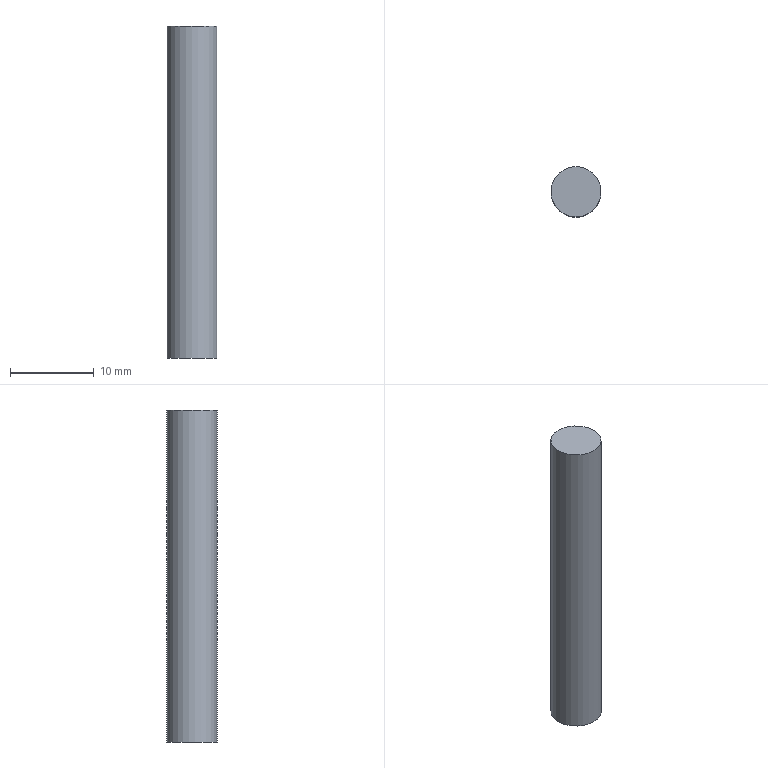Part | STEP file | Tube feed_id18_x_t | 1 solid | 3 faces | box 6 x 6 x 39.6 mm | volume 1120 mm3 | plane 2 | cylinder 1 | commonest cylinder face diameters 6 x1
STEP:
#1=CARTESIAN_POINT('',(0.,0.,0.));
#2=DIRECTION('',(0.,0.,1.));
#3=DIRECTION('',(1.,0.,0.));
#4=AXIS2_PLACEMENT_3D('',#1,#2,#3);
#5=CARTESIAN_POINT('',(-544.,16.556,-40.9));
#6=VERTEX_POINT('',#5);
#7=CARTESIAN_POINT('',(-544.,19.556,-40.9));
#8=DIRECTION('',(0.,0.,1.));
#9=DIRECTION('',(0.,-1.,0.));
#10=AXIS2_PLACEMENT_3D('',#7,#8,#9);
#11=CIRCLE('',#10,3.);
#12=CARTESIAN_POINT('',(-544.,19.556,-40.9));
#13=DIRECTION('',(0.,0.,1.));
#14=DIRECTION('',(1.,0.,0.));
#15=AXIS2_PLACEMENT_3D('',#12,#13,#14);
#16=CYLINDRICAL_SURFACE('',#15,3.);
#17=CARTESIAN_POINT('',(4.712,0.));
#18=DIRECTION('',(1.,0.));
#19=VECTOR('',#18,1.);
#20=LINE('',#17,#19);
#21=(GEOMETRIC_REPRESENTATION_CONTEXT(2)PARAMETRIC_REPRESENTATION_CONTEXT()REPRESENTATION_CONTEXT('',''));
#22=DEFINITIONAL_REPRESENTATION('',(#20),#21);
#23=PCURVE('',#16,#22);
#24=CARTESIAN_POINT('',(-544.,19.556,-40.9));
#25=DIRECTION('',(0.,0.,1.));
#26=DIRECTION('',(1.,0.,0.));
#27=AXIS2_PLACEMENT_3D('',#24,#25,#26);
#28=PLANE('',#27);
#29=CARTESIAN_POINT('',(0.,0.));
#30=DIRECTION('',(0.,-1.));
#31=AXIS2_PLACEMENT_2D('',#29,#30);
#32=CIRCLE('',#31,3.);
#33=(GEOMETRIC_REPRESENTATION_CONTEXT(2)PARAMETRIC_REPRESENTATION_CONTEXT()REPRESENTATION_CONTEXT('',''));
#34=DEFINITIONAL_REPRESENTATION('',(#32),#33);
#35=PCURVE('',#28,#34);
#36=SURFACE_CURVE('',#11,(#23,#35),.PCURVE_S1.);
#37=EDGE_CURVE('',#6,#6,#36,.T.);
#38=ORIENTED_EDGE('',*,*,#37,.T.);
#39=CARTESIAN_POINT('',(-544.,16.556,-1.3));
#40=VERTEX_POINT('',#39);
#41=CARTESIAN_POINT('',(-544.,16.556,-40.9));
#42=CARTESIAN_POINT('',(-544.,16.556,-1.3));
#43=B_SPLINE_CURVE_WITH_KNOTS('',1,(#41,#42),.UNSPECIFIED.,.F.,.F.,(2,2),(0.,39.6),.PIECEWISE_BEZIER_KNOTS.);
#44=CARTESIAN_POINT('',(10.996,0.));
#45=DIRECTION('',(0.,1.));
#46=VECTOR('',#45,1.);
#47=LINE('',#44,#46);
#48=(GEOMETRIC_REPRESENTATION_CONTEXT(2)PARAMETRIC_REPRESENTATION_CONTEXT()REPRESENTATION_CONTEXT('',''));
#49=DEFINITIONAL_REPRESENTATION('',(#47),#48);
#50=PCURVE('',#16,#49);
#51=CARTESIAN_POINT('',(4.712,0.));
#52=DIRECTION('',(0.,1.));
#53=VECTOR('',#52,1.);
#54=LINE('',#51,#53);
#55=(GEOMETRIC_REPRESENTATION_CONTEXT(2)PARAMETRIC_REPRESENTATION_CONTEXT()REPRESENTATION_CONTEXT('',''));
#56=DEFINITIONAL_REPRESENTATION('',(#54),#55);
#57=PCURVE('',#16,#56);
#58=SEAM_CURVE('',#43,(#50,#57),.PCURVE_S1.);
#59=EDGE_CURVE('',#6,#40,#58,.T.);
#60=ORIENTED_EDGE('',*,*,#59,.T.);
#61=CARTESIAN_POINT('',(-544.,19.556,-1.3));
#62=DIRECTION('',(0.,0.,1.));
#63=DIRECTION('',(0.,-1.,0.));
#64=AXIS2_PLACEMENT_3D('',#61,#62,#63);
#65=CIRCLE('',#64,3.);
#66=CARTESIAN_POINT('',(4.712,39.6));
#67=DIRECTION('',(1.,0.));
#68=VECTOR('',#67,1.);
#69=LINE('',#66,#68);
#70=(GEOMETRIC_REPRESENTATION_CONTEXT(2)PARAMETRIC_REPRESENTATION_CONTEXT()REPRESENTATION_CONTEXT('',''));
#71=DEFINITIONAL_REPRESENTATION('',(#69),#70);
#72=PCURVE('',#16,#71);
#73=CARTESIAN_POINT('',(-554.,29.736,-1.3));
#74=DIRECTION('',(0.,0.,1.));
#75=DIRECTION('',(0.,-1.,0.));
#76=AXIS2_PLACEMENT_3D('',#73,#74,#75);
#77=PLANE('',#76);
#78=CARTESIAN_POINT('',(10.18,10.));
#79=DIRECTION('',(1.,0.));
#80=AXIS2_PLACEMENT_2D('',#78,#79);
#81=CIRCLE('',#80,3.);
#82=(GEOMETRIC_REPRESENTATION_CONTEXT(2)PARAMETRIC_REPRESENTATION_CONTEXT()REPRESENTATION_CONTEXT('',''));
#83=DEFINITIONAL_REPRESENTATION('',(#81),#82);
#84=PCURVE('',#77,#83);
#85=SURFACE_CURVE('',#65,(#72,#84),.PCURVE_S1.);
#86=EDGE_CURVE('',#40,#40,#85,.T.);
#87=ORIENTED_EDGE('',*,*,#86,.F.);
#88=ORIENTED_EDGE('',*,*,#59,.F.);
#89=EDGE_LOOP('',(#38,#60,#87,#88));
#90=FACE_BOUND('',#89,.T.);
#91=ADVANCED_FACE('',(#90),#16,.T.);
#92=ORIENTED_EDGE('',*,*,#37,.F.);
#93=EDGE_LOOP('',(#92));
#94=FACE_BOUND('',#93,.T.);
#95=ADVANCED_FACE('',(#94),#28,.F.);
#96=ORIENTED_EDGE('',*,*,#86,.T.);
#97=EDGE_LOOP('',(#96));
#98=FACE_BOUND('',#97,.T.);
#99=ADVANCED_FACE('',(#98),#77,.T.);
#100=CLOSED_SHELL('',(#91,#95,#99));
#101=MANIFOLD_SOLID_BREP('',#100);
#102=(LENGTH_UNIT()NAMED_UNIT(*)SI_UNIT(.MILLI.,.METRE.));
#103=UNCERTAINTY_MEASURE_WITH_UNIT(LENGTH_MEASURE(0.00001),#102,'','');
#104=(NAMED_UNIT(*)PLANE_ANGLE_UNIT()SI_UNIT($,.RADIAN.));
#105=(NAMED_UNIT(*)SI_UNIT($,.STERADIAN.)SOLID_ANGLE_UNIT());
#106=(GEOMETRIC_REPRESENTATION_CONTEXT(3)GLOBAL_UNCERTAINTY_ASSIGNED_CONTEXT((#103))GLOBAL_UNIT_ASSIGNED_CONTEXT((#102,#104,#105))REPRESENTATION_CONTEXT('',''));
#107=ADVANCED_BREP_SHAPE_REPRESENTATION('',(#4,#101),#106);